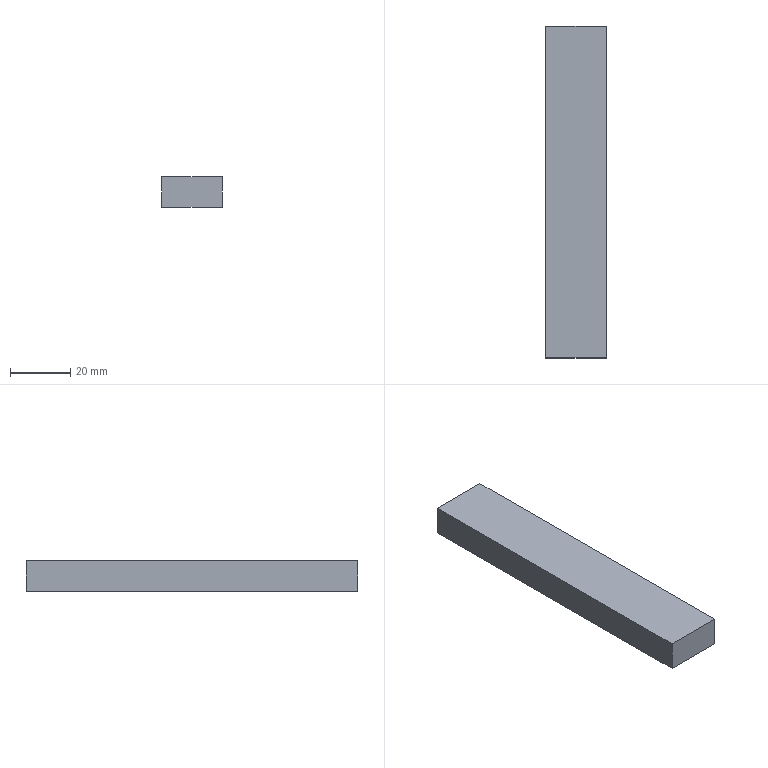Part | NX | features solid 2 | 1 solid | 6 faces | box 20 x 110 x 10 mm | volume 22000 mm3 | plane 6
STEP:
#1=CARTESIAN_POINT('',(-85.,417.,-83.));
#2=VERTEX_POINT('',#1);
#3=CARTESIAN_POINT('',(-65.,417.,-83.));
#4=VERTEX_POINT('',#3);
#5=CARTESIAN_POINT('',(-85.,417.,-83.));
#6=DIRECTION('',(1.,0.,0.));
#7=VECTOR('',#6,1000.);
#8=LINE('',#5,#7);
#9=EDGE_CURVE('',#2,#4,#8,.T.);
#10=ORIENTED_EDGE('',*,*,#9,.T.);
#11=CARTESIAN_POINT('',(-65.,417.,-73.));
#12=VERTEX_POINT('',#11);
#13=CARTESIAN_POINT('',(-65.,417.,27.));
#14=DIRECTION('',(0.,0.,-1.));
#15=VECTOR('',#14,1000.);
#16=LINE('',#13,#15);
#17=EDGE_CURVE('',#12,#4,#16,.T.);
#18=ORIENTED_EDGE('',*,*,#17,.F.);
#19=CARTESIAN_POINT('',(-85.,417.,-73.));
#20=VERTEX_POINT('',#19);
#21=CARTESIAN_POINT('',(-85.,417.,-73.));
#22=DIRECTION('',(-1.,0.,0.));
#23=VECTOR('',#22,1000.);
#24=LINE('',#21,#23);
#25=EDGE_CURVE('',#20,#12,#24,.F.);
#26=ORIENTED_EDGE('',*,*,#25,.F.);
#27=CARTESIAN_POINT('',(-85.,417.,27.));
#28=DIRECTION('',(0.,0.,-1.));
#29=VECTOR('',#28,1000.);
#30=LINE('',#27,#29);
#31=EDGE_CURVE('',#20,#2,#30,.T.);
#32=ORIENTED_EDGE('',*,*,#31,.T.);
#33=EDGE_LOOP('',(#10,#18,#26,#32));
#34=FACE_BOUND('',#33,.T.);
#35=CARTESIAN_POINT('',(-85.,417.,27.));
#36=DIRECTION('',(0.,-1.,0.));
#37=DIRECTION('',(0.,0.,-1.));
#38=AXIS2_PLACEMENT_3D('',#35,#36,#37);
#39=PLANE('',#38);
#40=ADVANCED_FACE('',(#34),#39,.T.);
#41=ORIENTED_EDGE('',*,*,#25,.T.);
#42=CARTESIAN_POINT('',(-65.,527.,-73.));
#43=VERTEX_POINT('',#42);
#44=CARTESIAN_POINT('',(-65.,427.,-73.));
#45=DIRECTION('',(0.,1.,0.));
#46=VECTOR('',#45,1000.);
#47=LINE('',#44,#46);
#48=EDGE_CURVE('',#12,#43,#47,.T.);
#49=ORIENTED_EDGE('',*,*,#48,.T.);
#50=CARTESIAN_POINT('',(-85.,527.,-73.));
#51=VERTEX_POINT('',#50);
#52=CARTESIAN_POINT('',(-85.,527.,-73.));
#53=DIRECTION('',(1.,0.,0.));
#54=VECTOR('',#53,1000.);
#55=LINE('',#52,#54);
#56=EDGE_CURVE('',#51,#43,#55,.T.);
#57=ORIENTED_EDGE('',*,*,#56,.F.);
#58=CARTESIAN_POINT('',(-85.,427.,-73.));
#59=DIRECTION('',(0.,1.,0.));
#60=VECTOR('',#59,1000.);
#61=LINE('',#58,#60);
#62=EDGE_CURVE('',#20,#51,#61,.T.);
#63=ORIENTED_EDGE('',*,*,#62,.F.);
#64=EDGE_LOOP('',(#41,#49,#57,#63));
#65=FACE_BOUND('',#64,.T.);
#66=CARTESIAN_POINT('',(-85.,427.,-73.));
#67=DIRECTION('',(0.,0.,-1.));
#68=DIRECTION('',(0.,1.,0.));
#69=AXIS2_PLACEMENT_3D('',#66,#67,#68);
#70=PLANE('',#69);
#71=ADVANCED_FACE('',(#65),#70,.F.);
#72=ORIENTED_EDGE('',*,*,#56,.T.);
#73=CARTESIAN_POINT('',(-65.,527.,-83.));
#74=VERTEX_POINT('',#73);
#75=CARTESIAN_POINT('',(-65.,527.,-73.));
#76=DIRECTION('',(0.,0.,-1.));
#77=VECTOR('',#76,1000.);
#78=LINE('',#75,#77);
#79=EDGE_CURVE('',#43,#74,#78,.T.);
#80=ORIENTED_EDGE('',*,*,#79,.T.);
#81=CARTESIAN_POINT('',(-85.,527.,-83.));
#82=VERTEX_POINT('',#81);
#83=CARTESIAN_POINT('',(-85.,527.,-83.));
#84=DIRECTION('',(1.,0.,0.));
#85=VECTOR('',#84,1000.);
#86=LINE('',#83,#85);
#87=EDGE_CURVE('',#82,#74,#86,.T.);
#88=ORIENTED_EDGE('',*,*,#87,.F.);
#89=CARTESIAN_POINT('',(-85.,527.,-73.));
#90=DIRECTION('',(0.,0.,-1.));
#91=VECTOR('',#90,1000.);
#92=LINE('',#89,#91);
#93=EDGE_CURVE('',#51,#82,#92,.T.);
#94=ORIENTED_EDGE('',*,*,#93,.F.);
#95=EDGE_LOOP('',(#72,#80,#88,#94));
#96=FACE_BOUND('',#95,.T.);
#97=CARTESIAN_POINT('',(-85.,527.,-73.));
#98=DIRECTION('',(0.,-1.,0.));
#99=DIRECTION('',(0.,0.,-1.));
#100=AXIS2_PLACEMENT_3D('',#97,#98,#99);
#101=PLANE('',#100);
#102=ADVANCED_FACE('',(#96),#101,.F.);
#103=CARTESIAN_POINT('',(-85.,427.,-83.));
#104=DIRECTION('',(0.,1.,0.));
#105=VECTOR('',#104,1000.);
#106=LINE('',#103,#105);
#107=EDGE_CURVE('',#2,#82,#106,.T.);
#108=ORIENTED_EDGE('',*,*,#107,.T.);
#109=ORIENTED_EDGE('',*,*,#87,.T.);
#110=CARTESIAN_POINT('',(-65.,427.,-83.));
#111=DIRECTION('',(0.,1.,0.));
#112=VECTOR('',#111,1000.);
#113=LINE('',#110,#112);
#114=EDGE_CURVE('',#4,#74,#113,.T.);
#115=ORIENTED_EDGE('',*,*,#114,.F.);
#116=ORIENTED_EDGE('',*,*,#9,.F.);
#117=EDGE_LOOP('',(#108,#109,#115,#116));
#118=FACE_BOUND('',#117,.T.);
#119=CARTESIAN_POINT('',(-85.,427.,-83.));
#120=DIRECTION('',(0.,0.,-1.));
#121=DIRECTION('',(0.,1.,0.));
#122=AXIS2_PLACEMENT_3D('',#119,#120,#121);
#123=PLANE('',#122);
#124=ADVANCED_FACE('',(#118),#123,.T.);
#125=ORIENTED_EDGE('',*,*,#79,.F.);
#126=ORIENTED_EDGE('',*,*,#48,.F.);
#127=ORIENTED_EDGE('',*,*,#17,.T.);
#128=ORIENTED_EDGE('',*,*,#114,.T.);
#129=EDGE_LOOP('',(#125,#126,#127,#128));
#130=FACE_BOUND('',#129,.T.);
#131=CARTESIAN_POINT('',(-65.,427.,-73.));
#132=DIRECTION('',(-1.,0.,0.));
#133=DIRECTION('',(0.,0.,-1.));
#134=AXIS2_PLACEMENT_3D('',#131,#132,#133);
#135=PLANE('',#134);
#136=ADVANCED_FACE('',(#130),#135,.F.);
#137=ORIENTED_EDGE('',*,*,#93,.T.);
#138=ORIENTED_EDGE('',*,*,#107,.F.);
#139=ORIENTED_EDGE('',*,*,#31,.F.);
#140=ORIENTED_EDGE('',*,*,#62,.T.);
#141=EDGE_LOOP('',(#137,#138,#139,#140));
#142=FACE_BOUND('',#141,.T.);
#143=CARTESIAN_POINT('',(-85.,427.,-73.));
#144=DIRECTION('',(-1.,0.,0.));
#145=DIRECTION('',(0.,0.,-1.));
#146=AXIS2_PLACEMENT_3D('',#143,#144,#145);
#147=PLANE('',#146);
#148=ADVANCED_FACE('',(#142),#147,.T.);
#149=CLOSED_SHELL('',(#40,#71,#102,#124,#136,#148));
#150=MANIFOLD_SOLID_BREP('',#149);
#151=(LENGTH_UNIT()NAMED_UNIT(*)SI_UNIT(.MILLI.,.METRE.));
#152=UNCERTAINTY_MEASURE_WITH_UNIT(LENGTH_MEASURE(0.00001),#151,'','');
#153=(NAMED_UNIT(*)PLANE_ANGLE_UNIT()SI_UNIT($,.RADIAN.));
#154=(NAMED_UNIT(*)SI_UNIT($,.STERADIAN.)SOLID_ANGLE_UNIT());
#155=(GEOMETRIC_REPRESENTATION_CONTEXT(3)GLOBAL_UNCERTAINTY_ASSIGNED_CONTEXT((#152))GLOBAL_UNIT_ASSIGNED_CONTEXT((#151,#153,#154))REPRESENTATION_CONTEXT('',''));
#156=ADVANCED_BREP_SHAPE_REPRESENTATION('',(#150),#155);